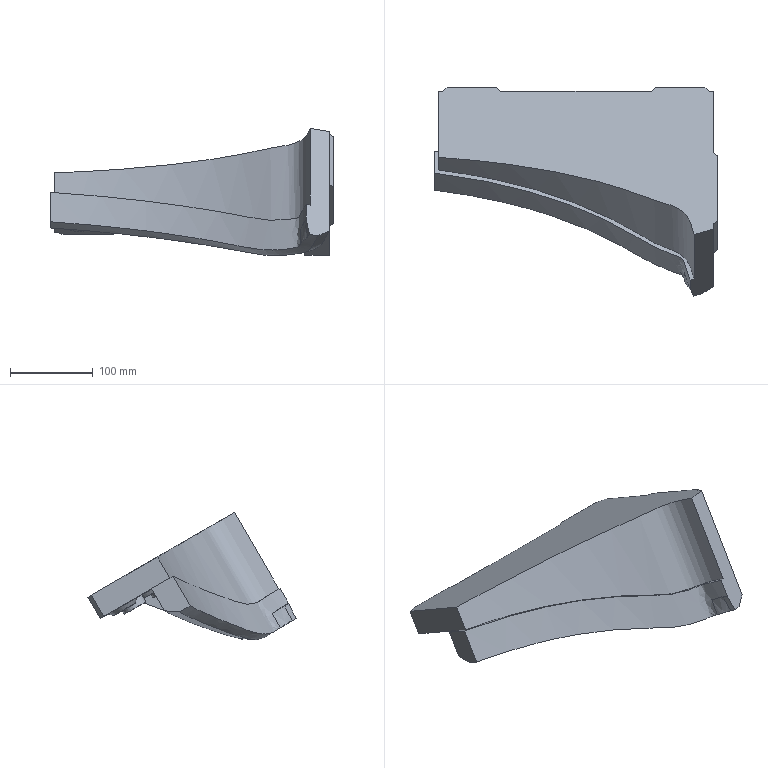Part | NX | features solid 2 | 1 solid | 45 faces | box 341.667 x 251.534 x 153.956 mm | volume 2359000 mm3 | plane 28 | spline 11 | cone 4 | cylinder 2 | commonest cylinder face diameters 30 x2